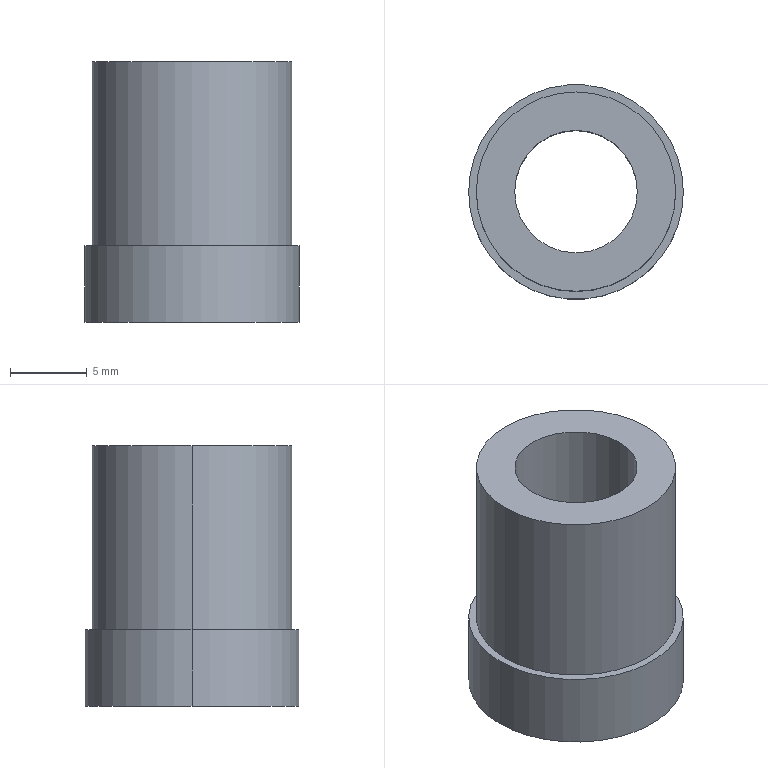Part | SolidWorks | features Extrusion 1, ICE 1 | 1 solid | 9 faces | box 14 x 14 x 17 mm | volume 1508 mm3 | cylinder 6 | plane 3 | commonest cylinder face diameters 8 x2 13 x2 14 x2
STEP:
#1=CARTESIAN_POINT('',(6.5,0.,17.));
#2=VERTEX_POINT('',#1);
#3=CARTESIAN_POINT('',(-6.5,0.,17.));
#4=VERTEX_POINT('',#3);
#5=CARTESIAN_POINT('',(0.,0.,17.));
#6=DIRECTION('',(0.,0.,1.));
#7=DIRECTION('',(1.,0.,0.));
#8=AXIS2_PLACEMENT_3D('',#5,#6,#7);
#9=CIRCLE('',#8,6.5);
#10=EDGE_CURVE('',#2,#4,#9,.T.);
#11=ORIENTED_EDGE('',*,*,#10,.F.);
#12=CARTESIAN_POINT('',(6.5,0.,5.));
#13=VERTEX_POINT('',#12);
#14=CARTESIAN_POINT('',(6.5,0.,17.));
#15=DIRECTION('',(0.,0.,-1.));
#16=VECTOR('',#15,1000.);
#17=LINE('',#14,#16);
#18=EDGE_CURVE('',#2,#13,#17,.T.);
#19=ORIENTED_EDGE('',*,*,#18,.T.);
#20=CARTESIAN_POINT('',(-6.5,0.,5.));
#21=VERTEX_POINT('',#20);
#22=CARTESIAN_POINT('',(0.,0.,5.));
#23=DIRECTION('',(0.,0.,1.));
#24=DIRECTION('',(1.,0.,0.));
#25=AXIS2_PLACEMENT_3D('',#22,#23,#24);
#26=CIRCLE('',#25,6.5);
#27=EDGE_CURVE('',#13,#21,#26,.T.);
#28=ORIENTED_EDGE('',*,*,#27,.T.);
#29=CARTESIAN_POINT('',(-6.5,0.,17.));
#30=DIRECTION('',(0.,0.,-1.));
#31=VECTOR('',#30,1000.);
#32=LINE('',#29,#31);
#33=EDGE_CURVE('',#4,#21,#32,.T.);
#34=ORIENTED_EDGE('',*,*,#33,.F.);
#35=EDGE_LOOP('',(#11,#19,#28,#34));
#36=FACE_OUTER_BOUND('',#35,.T.);
#37=CARTESIAN_POINT('',(0.,0.,17.));
#38=DIRECTION('',(0.,0.,-1.));
#39=DIRECTION('',(-1.,0.,0.));
#40=AXIS2_PLACEMENT_3D('',#37,#38,#39);
#41=CYLINDRICAL_SURFACE('',#40,6.5);
#42=ADVANCED_FACE('',(#36),#41,.T.);
#43=CARTESIAN_POINT('',(-4.,0.,17.));
#44=VERTEX_POINT('',#43);
#45=CARTESIAN_POINT('',(4.,0.,17.));
#46=VERTEX_POINT('',#45);
#47=CARTESIAN_POINT('',(0.,0.,17.));
#48=DIRECTION('',(0.,0.,1.));
#49=DIRECTION('',(1.,0.,0.));
#50=AXIS2_PLACEMENT_3D('',#47,#48,#49);
#51=CIRCLE('',#50,4.);
#52=EDGE_CURVE('',#44,#46,#51,.T.);
#53=ORIENTED_EDGE('',*,*,#52,.T.);
#54=CARTESIAN_POINT('',(4.,0.,0.));
#55=VERTEX_POINT('',#54);
#56=CARTESIAN_POINT('',(4.,0.,5.));
#57=DIRECTION('',(0.,0.,-1.));
#58=VECTOR('',#57,1000.);
#59=LINE('',#56,#58);
#60=EDGE_CURVE('',#46,#55,#59,.T.);
#61=ORIENTED_EDGE('',*,*,#60,.T.);
#62=CARTESIAN_POINT('',(-4.,0.,0.));
#63=VERTEX_POINT('',#62);
#64=CARTESIAN_POINT('',(0.,0.,0.));
#65=DIRECTION('',(0.,0.,1.));
#66=DIRECTION('',(1.,0.,0.));
#67=AXIS2_PLACEMENT_3D('',#64,#65,#66);
#68=CIRCLE('',#67,4.);
#69=EDGE_CURVE('',#63,#55,#68,.T.);
#70=ORIENTED_EDGE('',*,*,#69,.F.);
#71=CARTESIAN_POINT('',(-4.,0.,5.));
#72=DIRECTION('',(0.,0.,-1.));
#73=VECTOR('',#72,1000.);
#74=LINE('',#71,#73);
#75=EDGE_CURVE('',#44,#63,#74,.T.);
#76=ORIENTED_EDGE('',*,*,#75,.F.);
#77=EDGE_LOOP('',(#53,#61,#70,#76));
#78=FACE_OUTER_BOUND('',#77,.T.);
#79=CARTESIAN_POINT('',(0.,0.,5.));
#80=DIRECTION('',(0.,0.,-1.));
#81=DIRECTION('',(-1.,0.,0.));
#82=AXIS2_PLACEMENT_3D('',#79,#80,#81);
#83=CYLINDRICAL_SURFACE('',#82,4.);
#84=ADVANCED_FACE('',(#78),#83,.F.);
#85=CARTESIAN_POINT('',(7.,0.,5.));
#86=VERTEX_POINT('',#85);
#87=CARTESIAN_POINT('',(-7.,0.,5.));
#88=VERTEX_POINT('',#87);
#89=CARTESIAN_POINT('',(0.,0.,5.));
#90=DIRECTION('',(0.,0.,1.));
#91=DIRECTION('',(1.,0.,0.));
#92=AXIS2_PLACEMENT_3D('',#89,#90,#91);
#93=CIRCLE('',#92,7.);
#94=EDGE_CURVE('',#86,#88,#93,.T.);
#95=ORIENTED_EDGE('',*,*,#94,.F.);
#96=CARTESIAN_POINT('',(7.,0.,0.));
#97=VERTEX_POINT('',#96);
#98=CARTESIAN_POINT('',(7.,0.,5.));
#99=DIRECTION('',(0.,0.,-1.));
#100=VECTOR('',#99,1000.);
#101=LINE('',#98,#100);
#102=EDGE_CURVE('',#86,#97,#101,.T.);
#103=ORIENTED_EDGE('',*,*,#102,.T.);
#104=CARTESIAN_POINT('',(-7.,0.,0.));
#105=VERTEX_POINT('',#104);
#106=CARTESIAN_POINT('',(0.,0.,0.));
#107=DIRECTION('',(0.,0.,1.));
#108=DIRECTION('',(1.,0.,0.));
#109=AXIS2_PLACEMENT_3D('',#106,#107,#108);
#110=CIRCLE('',#109,7.);
#111=EDGE_CURVE('',#97,#105,#110,.T.);
#112=ORIENTED_EDGE('',*,*,#111,.T.);
#113=CARTESIAN_POINT('',(-7.,0.,5.));
#114=DIRECTION('',(0.,0.,-1.));
#115=VECTOR('',#114,1000.);
#116=LINE('',#113,#115);
#117=EDGE_CURVE('',#88,#105,#116,.T.);
#118=ORIENTED_EDGE('',*,*,#117,.F.);
#119=EDGE_LOOP('',(#95,#103,#112,#118));
#120=FACE_OUTER_BOUND('',#119,.T.);
#121=CARTESIAN_POINT('',(0.,0.,5.));
#122=DIRECTION('',(0.,0.,-1.));
#123=DIRECTION('',(-1.,0.,0.));
#124=AXIS2_PLACEMENT_3D('',#121,#122,#123);
#125=CYLINDRICAL_SURFACE('',#124,7.);
#126=ADVANCED_FACE('',(#120),#125,.T.);
#127=CARTESIAN_POINT('',(0.,0.,5.));
#128=DIRECTION('',(0.,0.,1.));
#129=DIRECTION('',(1.,0.,0.));
#130=AXIS2_PLACEMENT_3D('',#127,#128,#129);
#131=CIRCLE('',#130,6.5);
#132=EDGE_CURVE('',#21,#13,#131,.T.);
#133=ORIENTED_EDGE('',*,*,#132,.F.);
#134=ORIENTED_EDGE('',*,*,#27,.F.);
#135=EDGE_LOOP('',(#133,#134));
#136=FACE_BOUND('',#135,.T.);
#137=CARTESIAN_POINT('',(0.,0.,5.));
#138=DIRECTION('',(0.,0.,1.));
#139=DIRECTION('',(1.,0.,0.));
#140=AXIS2_PLACEMENT_3D('',#137,#138,#139);
#141=CIRCLE('',#140,7.);
#142=EDGE_CURVE('',#88,#86,#141,.T.);
#143=ORIENTED_EDGE('',*,*,#142,.T.);
#144=ORIENTED_EDGE('',*,*,#94,.T.);
#145=EDGE_LOOP('',(#143,#144));
#146=FACE_OUTER_BOUND('',#145,.T.);
#147=CARTESIAN_POINT('',(0.,0.,5.));
#148=DIRECTION('',(0.,0.,1.));
#149=DIRECTION('',(1.,0.,0.));
#150=AXIS2_PLACEMENT_3D('',#147,#148,#149);
#151=PLANE('',#150);
#152=ADVANCED_FACE('',(#136,#146),#151,.T.);
#153=CARTESIAN_POINT('',(0.,0.,0.));
#154=DIRECTION('',(0.,0.,1.));
#155=DIRECTION('',(1.,0.,0.));
#156=AXIS2_PLACEMENT_3D('',#153,#154,#155);
#157=CIRCLE('',#156,7.);
#158=EDGE_CURVE('',#105,#97,#157,.T.);
#159=ORIENTED_EDGE('',*,*,#158,.F.);
#160=ORIENTED_EDGE('',*,*,#111,.F.);
#161=EDGE_LOOP('',(#159,#160));
#162=FACE_OUTER_BOUND('',#161,.T.);
#163=ORIENTED_EDGE('',*,*,#69,.T.);
#164=CARTESIAN_POINT('',(0.,0.,0.));
#165=DIRECTION('',(0.,0.,1.));
#166=DIRECTION('',(1.,0.,0.));
#167=AXIS2_PLACEMENT_3D('',#164,#165,#166);
#168=CIRCLE('',#167,4.);
#169=EDGE_CURVE('',#55,#63,#168,.T.);
#170=ORIENTED_EDGE('',*,*,#169,.T.);
#171=EDGE_LOOP('',(#163,#170));
#172=FACE_BOUND('',#171,.T.);
#173=CARTESIAN_POINT('',(0.,0.,0.));
#174=DIRECTION('',(0.,0.,1.));
#175=DIRECTION('',(1.,0.,0.));
#176=AXIS2_PLACEMENT_3D('',#173,#174,#175);
#177=PLANE('',#176);
#178=ADVANCED_FACE('',(#162,#172),#177,.F.);
#179=ORIENTED_EDGE('',*,*,#102,.F.);
#180=ORIENTED_EDGE('',*,*,#142,.F.);
#181=ORIENTED_EDGE('',*,*,#117,.T.);
#182=ORIENTED_EDGE('',*,*,#158,.T.);
#183=EDGE_LOOP('',(#179,#180,#181,#182));
#184=FACE_OUTER_BOUND('',#183,.T.);
#185=CARTESIAN_POINT('',(0.,0.,5.));
#186=DIRECTION('',(0.,0.,-1.));
#187=DIRECTION('',(-1.,0.,0.));
#188=AXIS2_PLACEMENT_3D('',#185,#186,#187);
#189=CYLINDRICAL_SURFACE('',#188,7.);
#190=ADVANCED_FACE('',(#184),#189,.T.);
#191=ORIENTED_EDGE('',*,*,#60,.F.);
#192=CARTESIAN_POINT('',(0.,0.,17.));
#193=DIRECTION('',(0.,0.,1.));
#194=DIRECTION('',(1.,0.,0.));
#195=AXIS2_PLACEMENT_3D('',#192,#193,#194);
#196=CIRCLE('',#195,4.);
#197=EDGE_CURVE('',#46,#44,#196,.T.);
#198=ORIENTED_EDGE('',*,*,#197,.T.);
#199=ORIENTED_EDGE('',*,*,#75,.T.);
#200=ORIENTED_EDGE('',*,*,#169,.F.);
#201=EDGE_LOOP('',(#191,#198,#199,#200));
#202=FACE_OUTER_BOUND('',#201,.T.);
#203=CARTESIAN_POINT('',(0.,0.,5.));
#204=DIRECTION('',(0.,0.,-1.));
#205=DIRECTION('',(-1.,0.,0.));
#206=AXIS2_PLACEMENT_3D('',#203,#204,#205);
#207=CYLINDRICAL_SURFACE('',#206,4.);
#208=ADVANCED_FACE('',(#202),#207,.F.);
#209=CARTESIAN_POINT('',(0.,0.,17.));
#210=DIRECTION('',(0.,0.,1.));
#211=DIRECTION('',(1.,0.,0.));
#212=AXIS2_PLACEMENT_3D('',#209,#210,#211);
#213=CIRCLE('',#212,6.5);
#214=EDGE_CURVE('',#4,#2,#213,.T.);
#215=ORIENTED_EDGE('',*,*,#214,.T.);
#216=ORIENTED_EDGE('',*,*,#10,.T.);
#217=EDGE_LOOP('',(#215,#216));
#218=FACE_OUTER_BOUND('',#217,.T.);
#219=ORIENTED_EDGE('',*,*,#52,.F.);
#220=ORIENTED_EDGE('',*,*,#197,.F.);
#221=EDGE_LOOP('',(#219,#220));
#222=FACE_BOUND('',#221,.T.);
#223=CARTESIAN_POINT('',(0.,0.,17.));
#224=DIRECTION('',(0.,0.,1.));
#225=DIRECTION('',(1.,0.,0.));
#226=AXIS2_PLACEMENT_3D('',#223,#224,#225);
#227=PLANE('',#226);
#228=ADVANCED_FACE('',(#218,#222),#227,.T.);
#229=ORIENTED_EDGE('',*,*,#18,.F.);
#230=ORIENTED_EDGE('',*,*,#214,.F.);
#231=ORIENTED_EDGE('',*,*,#33,.T.);
#232=ORIENTED_EDGE('',*,*,#132,.T.);
#233=EDGE_LOOP('',(#229,#230,#231,#232));
#234=FACE_OUTER_BOUND('',#233,.T.);
#235=CARTESIAN_POINT('',(0.,0.,17.));
#236=DIRECTION('',(0.,0.,-1.));
#237=DIRECTION('',(-1.,0.,0.));
#238=AXIS2_PLACEMENT_3D('',#235,#236,#237);
#239=CYLINDRICAL_SURFACE('',#238,6.5);
#240=ADVANCED_FACE('',(#234),#239,.T.);
#241=CLOSED_SHELL('',(#42,#84,#126,#152,#178,#190,#208,#228,#240));
#242=MANIFOLD_SOLID_BREP('',#241);
#243=CARTESIAN_POINT('',(0.,0.,0.));
#244=DIRECTION('',(0.,0.,1.));
#245=DIRECTION('',(1.,0.,0.));
#246=AXIS2_PLACEMENT_3D('',#243,#244,#245);
#247=(LENGTH_UNIT()NAMED_UNIT(*)SI_UNIT(.MILLI.,.METRE.));
#248=UNCERTAINTY_MEASURE_WITH_UNIT(LENGTH_MEASURE(0.00001),#247,'','');
#249=(NAMED_UNIT(*)PLANE_ANGLE_UNIT()SI_UNIT($,.RADIAN.));
#250=(NAMED_UNIT(*)SI_UNIT($,.STERADIAN.)SOLID_ANGLE_UNIT());
#251=(GEOMETRIC_REPRESENTATION_CONTEXT(3)GLOBAL_UNCERTAINTY_ASSIGNED_CONTEXT((#248))GLOBAL_UNIT_ASSIGNED_CONTEXT((#247,#249,#250))REPRESENTATION_CONTEXT('',''));
#252=ADVANCED_BREP_SHAPE_REPRESENTATION('',(#242,#246),#251);